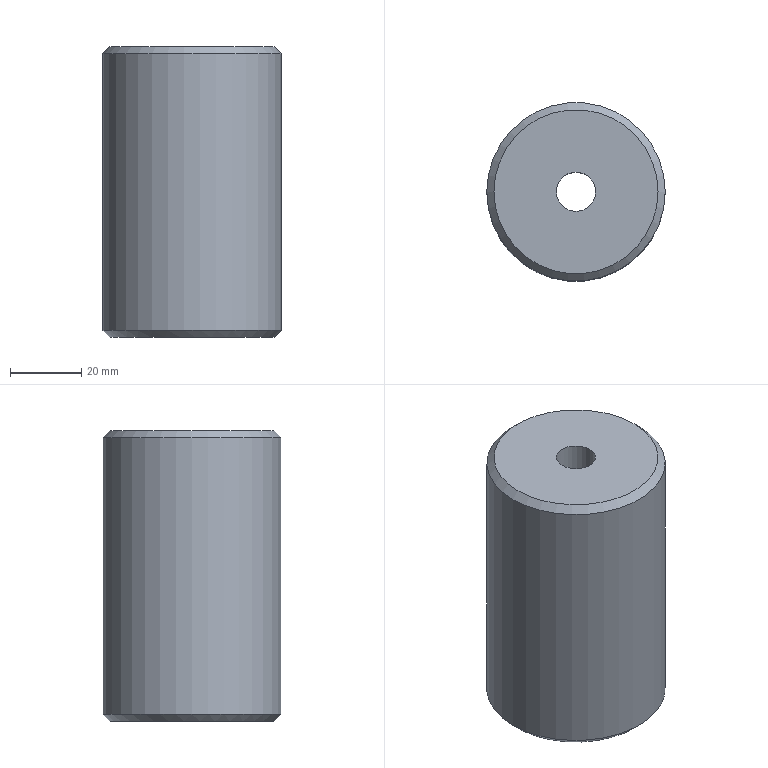Part | NX | features LIN_SOLID_COLOR 2 | 1 solid | 8 faces | box 50 x 50 x 81.5 mm | volume 143457 mm3 | cylinder 3 | plane 3 | cone 2 | commonest cylinder face diameters 11 x1 18 x1 50 x1
STEP:
#1=CARTESIAN_POINT('',(-59.,-200.,88.));
#2=VERTEX_POINT('',#1);
#3=CARTESIAN_POINT('',(-34.,-200.,88.));
#4=DIRECTION('',(0.,0.,-1.));
#5=DIRECTION('',(-1.,0.,0.));
#6=AXIS2_PLACEMENT_3D('',#3,#4,#5);
#7=CIRCLE('',#6,25.);
#8=EDGE_CURVE('',#2,#2,#7,.T.);
#9=ORIENTED_EDGE('',*,*,#8,.T.);
#10=EDGE_LOOP('',(#9));
#11=FACE_BOUND('',#10,.T.);
#12=CARTESIAN_POINT('',(-59.,-200.,10.5));
#13=VERTEX_POINT('',#12);
#14=CARTESIAN_POINT('',(-34.,-200.,10.5));
#15=DIRECTION('',(0.,0.,-1.));
#16=DIRECTION('',(-1.,0.,0.));
#17=AXIS2_PLACEMENT_3D('',#14,#15,#16);
#18=CIRCLE('',#17,25.);
#19=EDGE_CURVE('',#13,#13,#18,.F.);
#20=ORIENTED_EDGE('',*,*,#19,.T.);
#21=EDGE_LOOP('',(#20));
#22=FACE_BOUND('',#21,.T.);
#23=CARTESIAN_POINT('',(-34.,-200.,21.5));
#24=DIRECTION('',(0.,0.,1.));
#25=DIRECTION('',(1.,0.,0.));
#26=AXIS2_PLACEMENT_3D('',#23,#24,#25);
#27=CYLINDRICAL_SURFACE('',#26,25.);
#28=ADVANCED_FACE('',(#11,#22),#27,.T.);
#29=CARTESIAN_POINT('',(-11.,-200.,8.5));
#30=VERTEX_POINT('',#29);
#31=CARTESIAN_POINT('',(-34.,-200.,8.5));
#32=DIRECTION('',(0.,0.,1.));
#33=DIRECTION('',(1.,0.,0.));
#34=AXIS2_PLACEMENT_3D('',#31,#32,#33);
#35=CIRCLE('',#34,23.);
#36=EDGE_CURVE('',#30,#30,#35,.F.);
#37=ORIENTED_EDGE('',*,*,#36,.T.);
#38=EDGE_LOOP('',(#37));
#39=FACE_BOUND('',#38,.T.);
#40=CARTESIAN_POINT('',(-25.,-200.,8.5));
#41=VERTEX_POINT('',#40);
#42=CARTESIAN_POINT('',(-34.,-200.,8.5));
#43=DIRECTION('',(0.,0.,1.));
#44=DIRECTION('',(1.,0.,0.));
#45=AXIS2_PLACEMENT_3D('',#42,#43,#44);
#46=CIRCLE('',#45,9.);
#47=EDGE_CURVE('',#41,#41,#46,.F.);
#48=ORIENTED_EDGE('',*,*,#47,.F.);
#49=EDGE_LOOP('',(#48));
#50=FACE_BOUND('',#49,.T.);
#51=CARTESIAN_POINT('',(-34.,-200.,8.5));
#52=DIRECTION('',(0.,0.,1.));
#53=DIRECTION('',(1.,0.,0.));
#54=AXIS2_PLACEMENT_3D('',#51,#52,#53);
#55=PLANE('',#54);
#56=ADVANCED_FACE('',(#39,#50),#55,.F.);
#57=CARTESIAN_POINT('',(-11.,-200.,90.));
#58=VERTEX_POINT('',#57);
#59=CARTESIAN_POINT('',(-34.,-200.,90.));
#60=DIRECTION('',(0.,0.,1.));
#61=DIRECTION('',(1.,0.,0.));
#62=AXIS2_PLACEMENT_3D('',#59,#60,#61);
#63=CIRCLE('',#62,23.);
#64=EDGE_CURVE('',#58,#58,#63,.T.);
#65=ORIENTED_EDGE('',*,*,#64,.T.);
#66=EDGE_LOOP('',(#65));
#67=FACE_BOUND('',#66,.T.);
#68=CARTESIAN_POINT('',(-28.5,-200.,90.));
#69=VERTEX_POINT('',#68);
#70=CARTESIAN_POINT('',(-34.,-200.,90.));
#71=DIRECTION('',(0.,0.,1.));
#72=DIRECTION('',(1.,0.,0.));
#73=AXIS2_PLACEMENT_3D('',#70,#71,#72);
#74=CIRCLE('',#73,5.5);
#75=EDGE_CURVE('',#69,#69,#74,.F.);
#76=ORIENTED_EDGE('',*,*,#75,.T.);
#77=EDGE_LOOP('',(#76));
#78=FACE_BOUND('',#77,.T.);
#79=CARTESIAN_POINT('',(1103.,40.,90.));
#80=DIRECTION('',(0.,0.,1.));
#81=DIRECTION('',(1.,0.,0.));
#82=AXIS2_PLACEMENT_3D('',#79,#80,#81);
#83=PLANE('',#82);
#84=ADVANCED_FACE('',(#67,#78),#83,.T.);
#85=CARTESIAN_POINT('',(-28.5,-200.,60.));
#86=VERTEX_POINT('',#85);
#87=CARTESIAN_POINT('',(-34.,-200.,60.));
#88=DIRECTION('',(0.,0.,1.));
#89=DIRECTION('',(1.,0.,0.));
#90=AXIS2_PLACEMENT_3D('',#87,#88,#89);
#91=CIRCLE('',#90,5.5);
#92=EDGE_CURVE('',#86,#86,#91,.F.);
#93=ORIENTED_EDGE('',*,*,#92,.T.);
#94=EDGE_LOOP('',(#93));
#95=FACE_BOUND('',#94,.T.);
#96=ORIENTED_EDGE('',*,*,#75,.F.);
#97=EDGE_LOOP('',(#96));
#98=FACE_BOUND('',#97,.T.);
#99=CARTESIAN_POINT('',(-34.,-200.,90.));
#100=DIRECTION('',(0.,0.,-1.));
#101=DIRECTION('',(1.,0.,0.));
#102=AXIS2_PLACEMENT_3D('',#99,#100,#101);
#103=CYLINDRICAL_SURFACE('',#102,5.5);
#104=ADVANCED_FACE('',(#95,#98),#103,.F.);
#105=CARTESIAN_POINT('',(-25.,-200.,60.));
#106=VERTEX_POINT('',#105);
#107=CARTESIAN_POINT('',(-34.,-200.,60.));
#108=DIRECTION('',(0.,0.,1.));
#109=DIRECTION('',(1.,0.,0.));
#110=AXIS2_PLACEMENT_3D('',#107,#108,#109);
#111=CIRCLE('',#110,9.);
#112=EDGE_CURVE('',#106,#106,#111,.T.);
#113=ORIENTED_EDGE('',*,*,#112,.F.);
#114=EDGE_LOOP('',(#113));
#115=FACE_BOUND('',#114,.T.);
#116=ORIENTED_EDGE('',*,*,#92,.F.);
#117=EDGE_LOOP('',(#116));
#118=FACE_BOUND('',#117,.T.);
#119=CARTESIAN_POINT('',(-34.,-200.,60.));
#120=DIRECTION('',(0.,0.,1.));
#121=DIRECTION('',(1.,0.,0.));
#122=AXIS2_PLACEMENT_3D('',#119,#120,#121);
#123=PLANE('',#122);
#124=ADVANCED_FACE('',(#115,#118),#123,.F.);
#125=ORIENTED_EDGE('',*,*,#47,.T.);
#126=EDGE_LOOP('',(#125));
#127=FACE_BOUND('',#126,.T.);
#128=ORIENTED_EDGE('',*,*,#112,.T.);
#129=EDGE_LOOP('',(#128));
#130=FACE_BOUND('',#129,.T.);
#131=CARTESIAN_POINT('',(-34.,-200.,70.));
#132=DIRECTION('',(0.,0.,-1.));
#133=DIRECTION('',(1.,0.,0.));
#134=AXIS2_PLACEMENT_3D('',#131,#132,#133);
#135=CYLINDRICAL_SURFACE('',#134,9.);
#136=ADVANCED_FACE('',(#127,#130),#135,.F.);
#137=ORIENTED_EDGE('',*,*,#64,.F.);
#138=EDGE_LOOP('',(#137));
#139=FACE_BOUND('',#138,.T.);
#140=ORIENTED_EDGE('',*,*,#8,.F.);
#141=EDGE_LOOP('',(#140));
#142=FACE_BOUND('',#141,.T.);
#143=CARTESIAN_POINT('',(-34.,-200.,88.));
#144=DIRECTION('',(0.,0.,-1.));
#145=DIRECTION('',(-1.,0.,0.));
#146=AXIS2_PLACEMENT_3D('',#143,#144,#145);
#147=CONICAL_SURFACE('',#146,25.,0.7854);
#148=ADVANCED_FACE('',(#139,#142),#147,.T.);
#149=ORIENTED_EDGE('',*,*,#19,.F.);
#150=EDGE_LOOP('',(#149));
#151=FACE_BOUND('',#150,.T.);
#152=ORIENTED_EDGE('',*,*,#36,.F.);
#153=EDGE_LOOP('',(#152));
#154=FACE_BOUND('',#153,.T.);
#155=CARTESIAN_POINT('',(-34.,-200.,8.5));
#156=DIRECTION('',(0.,0.,1.));
#157=DIRECTION('',(1.,0.,0.));
#158=AXIS2_PLACEMENT_3D('',#155,#156,#157);
#159=CONICAL_SURFACE('',#158,23.,0.7854);
#160=ADVANCED_FACE('',(#151,#154),#159,.T.);
#161=CLOSED_SHELL('',(#28,#56,#84,#104,#124,#136,#148,#160));
#162=MANIFOLD_SOLID_BREP('',#161);
#163=(LENGTH_UNIT()NAMED_UNIT(*)SI_UNIT(.MILLI.,.METRE.));
#164=UNCERTAINTY_MEASURE_WITH_UNIT(LENGTH_MEASURE(0.00001),#163,'','');
#165=(NAMED_UNIT(*)PLANE_ANGLE_UNIT()SI_UNIT($,.RADIAN.));
#166=(NAMED_UNIT(*)SI_UNIT($,.STERADIAN.)SOLID_ANGLE_UNIT());
#167=(GEOMETRIC_REPRESENTATION_CONTEXT(3)GLOBAL_UNCERTAINTY_ASSIGNED_CONTEXT((#164))GLOBAL_UNIT_ASSIGNED_CONTEXT((#163,#165,#166))REPRESENTATION_CONTEXT('',''));
#168=ADVANCED_BREP_SHAPE_REPRESENTATION('',(#162),#167);